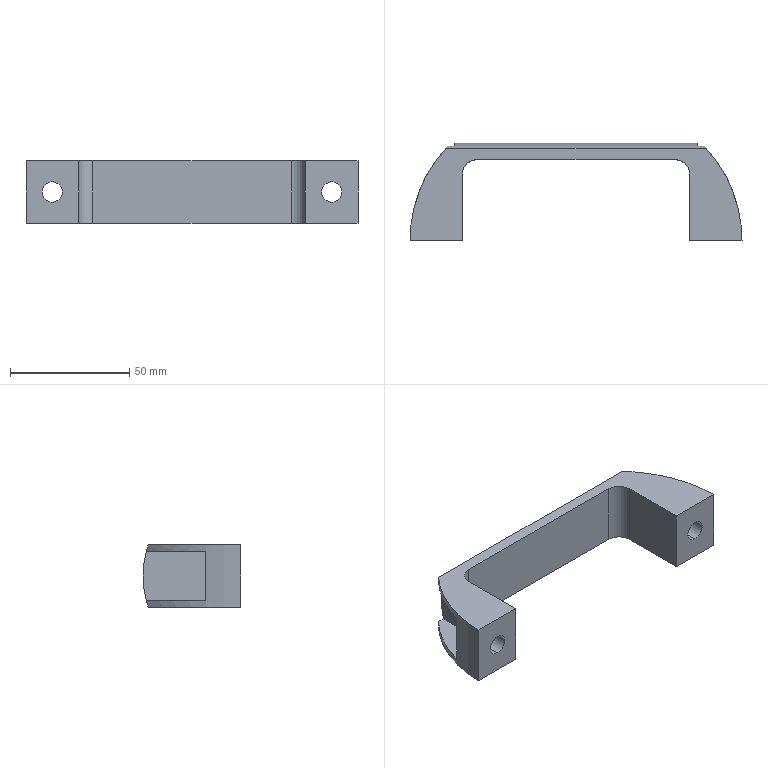Part | STEP file | UPCN26-B plastic handle | 1 solid | 30 faces | box 139 x 41 x 26 mm | volume 36631 mm3 | plane 17 | cylinder 13 | commonest cylinder face diameters 8.5 x4 13.3 x4 12 x2 115.6 x2 82 x1